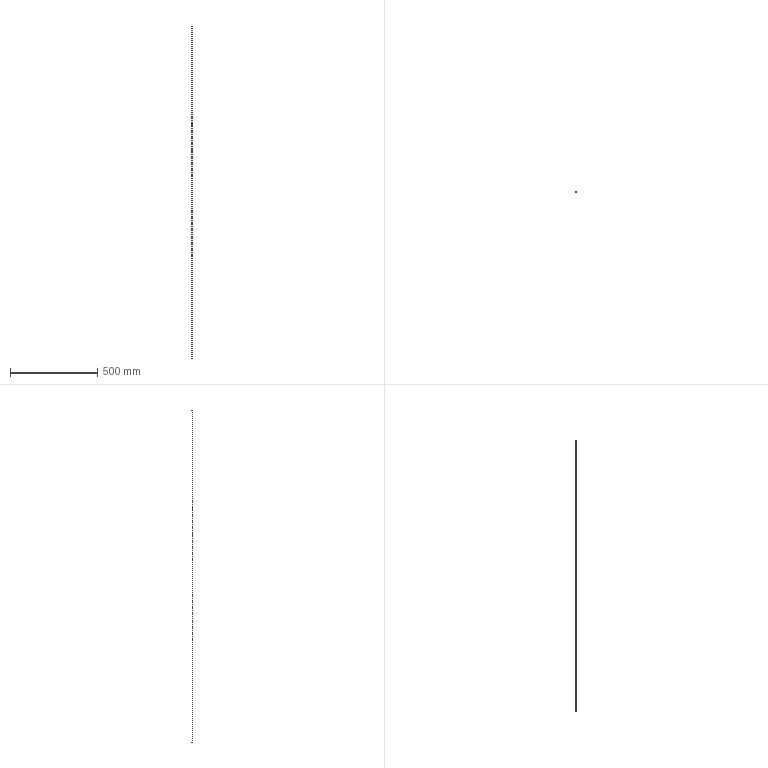Part | SolidWorks | features Extrusion 1 | 1 solid | 6 faces | box 0.15 x 0.15 x 1900 mm | volume 10.259 mm3 | cylinder 4 | plane 2 | commonest cylinder face diameters 0.125 x2 0.15 x2
STEP:
#1=CARTESIAN_POINT('',(-0.0625,0.,1900.));
#2=VERTEX_POINT('',#1);
#3=CARTESIAN_POINT('',(0.0625,0.,1900.));
#4=VERTEX_POINT('',#3);
#5=CARTESIAN_POINT('',(0.,0.,1900.));
#6=DIRECTION('',(0.,0.,1.));
#7=DIRECTION('',(1.,0.,0.));
#8=AXIS2_PLACEMENT_3D('',#5,#6,#7);
#9=CIRCLE('',#8,0.0625);
#10=EDGE_CURVE('',#2,#4,#9,.T.);
#11=ORIENTED_EDGE('',*,*,#10,.T.);
#12=CARTESIAN_POINT('',(0.0625,0.,0.));
#13=VERTEX_POINT('',#12);
#14=CARTESIAN_POINT('',(0.0625,0.,1900.));
#15=DIRECTION('',(0.,0.,-1.));
#16=VECTOR('',#15,1000.);
#17=LINE('',#14,#16);
#18=EDGE_CURVE('',#4,#13,#17,.T.);
#19=ORIENTED_EDGE('',*,*,#18,.T.);
#20=CARTESIAN_POINT('',(-0.0625,0.,0.));
#21=VERTEX_POINT('',#20);
#22=CARTESIAN_POINT('',(0.,0.,0.));
#23=DIRECTION('',(0.,0.,1.));
#24=DIRECTION('',(1.,0.,0.));
#25=AXIS2_PLACEMENT_3D('',#22,#23,#24);
#26=CIRCLE('',#25,0.0625);
#27=EDGE_CURVE('',#21,#13,#26,.T.);
#28=ORIENTED_EDGE('',*,*,#27,.F.);
#29=CARTESIAN_POINT('',(-0.0625,0.,1900.));
#30=DIRECTION('',(0.,0.,-1.));
#31=VECTOR('',#30,1000.);
#32=LINE('',#29,#31);
#33=EDGE_CURVE('',#2,#21,#32,.T.);
#34=ORIENTED_EDGE('',*,*,#33,.F.);
#35=EDGE_LOOP('',(#11,#19,#28,#34));
#36=FACE_OUTER_BOUND('',#35,.T.);
#37=CARTESIAN_POINT('',(0.,0.,1900.));
#38=DIRECTION('',(0.,0.,-1.));
#39=DIRECTION('',(-1.,0.,0.));
#40=AXIS2_PLACEMENT_3D('',#37,#38,#39);
#41=CYLINDRICAL_SURFACE('',#40,0.0625);
#42=ADVANCED_FACE('',(#36),#41,.F.);
#43=CARTESIAN_POINT('',(0.075,0.,1900.));
#44=VERTEX_POINT('',#43);
#45=CARTESIAN_POINT('',(-0.075,0.,1900.));
#46=VERTEX_POINT('',#45);
#47=CARTESIAN_POINT('',(0.,0.,1900.));
#48=DIRECTION('',(0.,0.,1.));
#49=DIRECTION('',(1.,0.,0.));
#50=AXIS2_PLACEMENT_3D('',#47,#48,#49);
#51=CIRCLE('',#50,0.075);
#52=EDGE_CURVE('',#44,#46,#51,.T.);
#53=ORIENTED_EDGE('',*,*,#52,.F.);
#54=CARTESIAN_POINT('',(0.075,0.,0.));
#55=VERTEX_POINT('',#54);
#56=CARTESIAN_POINT('',(0.075,0.,1900.));
#57=DIRECTION('',(0.,0.,-1.));
#58=VECTOR('',#57,1000.);
#59=LINE('',#56,#58);
#60=EDGE_CURVE('',#44,#55,#59,.T.);
#61=ORIENTED_EDGE('',*,*,#60,.T.);
#62=CARTESIAN_POINT('',(-0.075,0.,0.));
#63=VERTEX_POINT('',#62);
#64=CARTESIAN_POINT('',(0.,0.,0.));
#65=DIRECTION('',(0.,0.,1.));
#66=DIRECTION('',(1.,0.,0.));
#67=AXIS2_PLACEMENT_3D('',#64,#65,#66);
#68=CIRCLE('',#67,0.075);
#69=EDGE_CURVE('',#55,#63,#68,.T.);
#70=ORIENTED_EDGE('',*,*,#69,.T.);
#71=CARTESIAN_POINT('',(-0.075,0.,1900.));
#72=DIRECTION('',(0.,0.,-1.));
#73=VECTOR('',#72,1000.);
#74=LINE('',#71,#73);
#75=EDGE_CURVE('',#46,#63,#74,.T.);
#76=ORIENTED_EDGE('',*,*,#75,.F.);
#77=EDGE_LOOP('',(#53,#61,#70,#76));
#78=FACE_OUTER_BOUND('',#77,.T.);
#79=CARTESIAN_POINT('',(0.,0.,1900.));
#80=DIRECTION('',(0.,0.,-1.));
#81=DIRECTION('',(-1.,0.,0.));
#82=AXIS2_PLACEMENT_3D('',#79,#80,#81);
#83=CYLINDRICAL_SURFACE('',#82,0.075);
#84=ADVANCED_FACE('',(#78),#83,.T.);
#85=CARTESIAN_POINT('',(0.,0.,1900.));
#86=DIRECTION('',(0.,0.,1.));
#87=DIRECTION('',(1.,0.,0.));
#88=AXIS2_PLACEMENT_3D('',#85,#86,#87);
#89=CIRCLE('',#88,0.075);
#90=EDGE_CURVE('',#46,#44,#89,.T.);
#91=ORIENTED_EDGE('',*,*,#90,.T.);
#92=ORIENTED_EDGE('',*,*,#52,.T.);
#93=EDGE_LOOP('',(#91,#92));
#94=FACE_OUTER_BOUND('',#93,.T.);
#95=ORIENTED_EDGE('',*,*,#10,.F.);
#96=CARTESIAN_POINT('',(0.,0.,1900.));
#97=DIRECTION('',(0.,0.,1.));
#98=DIRECTION('',(1.,0.,0.));
#99=AXIS2_PLACEMENT_3D('',#96,#97,#98);
#100=CIRCLE('',#99,0.0625);
#101=EDGE_CURVE('',#4,#2,#100,.T.);
#102=ORIENTED_EDGE('',*,*,#101,.F.);
#103=EDGE_LOOP('',(#95,#102));
#104=FACE_BOUND('',#103,.T.);
#105=CARTESIAN_POINT('',(0.,0.,1900.));
#106=DIRECTION('',(0.,0.,1.));
#107=DIRECTION('',(1.,0.,0.));
#108=AXIS2_PLACEMENT_3D('',#105,#106,#107);
#109=PLANE('',#108);
#110=ADVANCED_FACE('',(#94,#104),#109,.T.);
#111=CARTESIAN_POINT('',(0.,0.,0.));
#112=DIRECTION('',(0.,0.,1.));
#113=DIRECTION('',(1.,0.,0.));
#114=AXIS2_PLACEMENT_3D('',#111,#112,#113);
#115=CIRCLE('',#114,0.075);
#116=EDGE_CURVE('',#63,#55,#115,.T.);
#117=ORIENTED_EDGE('',*,*,#116,.F.);
#118=ORIENTED_EDGE('',*,*,#69,.F.);
#119=EDGE_LOOP('',(#117,#118));
#120=FACE_OUTER_BOUND('',#119,.T.);
#121=ORIENTED_EDGE('',*,*,#27,.T.);
#122=CARTESIAN_POINT('',(0.,0.,0.));
#123=DIRECTION('',(0.,0.,1.));
#124=DIRECTION('',(1.,0.,0.));
#125=AXIS2_PLACEMENT_3D('',#122,#123,#124);
#126=CIRCLE('',#125,0.0625);
#127=EDGE_CURVE('',#13,#21,#126,.T.);
#128=ORIENTED_EDGE('',*,*,#127,.T.);
#129=EDGE_LOOP('',(#121,#128));
#130=FACE_BOUND('',#129,.T.);
#131=CARTESIAN_POINT('',(0.,0.,0.));
#132=DIRECTION('',(0.,0.,1.));
#133=DIRECTION('',(1.,0.,0.));
#134=AXIS2_PLACEMENT_3D('',#131,#132,#133);
#135=PLANE('',#134);
#136=ADVANCED_FACE('',(#120,#130),#135,.F.);
#137=ORIENTED_EDGE('',*,*,#60,.F.);
#138=ORIENTED_EDGE('',*,*,#90,.F.);
#139=ORIENTED_EDGE('',*,*,#75,.T.);
#140=ORIENTED_EDGE('',*,*,#116,.T.);
#141=EDGE_LOOP('',(#137,#138,#139,#140));
#142=FACE_OUTER_BOUND('',#141,.T.);
#143=CARTESIAN_POINT('',(0.,0.,1900.));
#144=DIRECTION('',(0.,0.,-1.));
#145=DIRECTION('',(-1.,0.,0.));
#146=AXIS2_PLACEMENT_3D('',#143,#144,#145);
#147=CYLINDRICAL_SURFACE('',#146,0.075);
#148=ADVANCED_FACE('',(#142),#147,.T.);
#149=ORIENTED_EDGE('',*,*,#18,.F.);
#150=ORIENTED_EDGE('',*,*,#101,.T.);
#151=ORIENTED_EDGE('',*,*,#33,.T.);
#152=ORIENTED_EDGE('',*,*,#127,.F.);
#153=EDGE_LOOP('',(#149,#150,#151,#152));
#154=FACE_OUTER_BOUND('',#153,.T.);
#155=CARTESIAN_POINT('',(0.,0.,1900.));
#156=DIRECTION('',(0.,0.,-1.));
#157=DIRECTION('',(-1.,0.,0.));
#158=AXIS2_PLACEMENT_3D('',#155,#156,#157);
#159=CYLINDRICAL_SURFACE('',#158,0.0625);
#160=ADVANCED_FACE('',(#154),#159,.F.);
#161=CLOSED_SHELL('',(#42,#84,#110,#136,#148,#160));
#162=MANIFOLD_SOLID_BREP('',#161);
#163=CARTESIAN_POINT('',(0.,0.,0.));
#164=DIRECTION('',(0.,0.,1.));
#165=DIRECTION('',(1.,0.,0.));
#166=AXIS2_PLACEMENT_3D('',#163,#164,#165);
#167=(LENGTH_UNIT()NAMED_UNIT(*)SI_UNIT(.MILLI.,.METRE.));
#168=UNCERTAINTY_MEASURE_WITH_UNIT(LENGTH_MEASURE(0.00001),#167,'','');
#169=(NAMED_UNIT(*)PLANE_ANGLE_UNIT()SI_UNIT($,.RADIAN.));
#170=(NAMED_UNIT(*)SI_UNIT($,.STERADIAN.)SOLID_ANGLE_UNIT());
#171=(GEOMETRIC_REPRESENTATION_CONTEXT(3)GLOBAL_UNCERTAINTY_ASSIGNED_CONTEXT((#168))GLOBAL_UNIT_ASSIGNED_CONTEXT((#167,#169,#170))REPRESENTATION_CONTEXT('',''));
#172=ADVANCED_BREP_SHAPE_REPRESENTATION('',(#162,#166),#171);